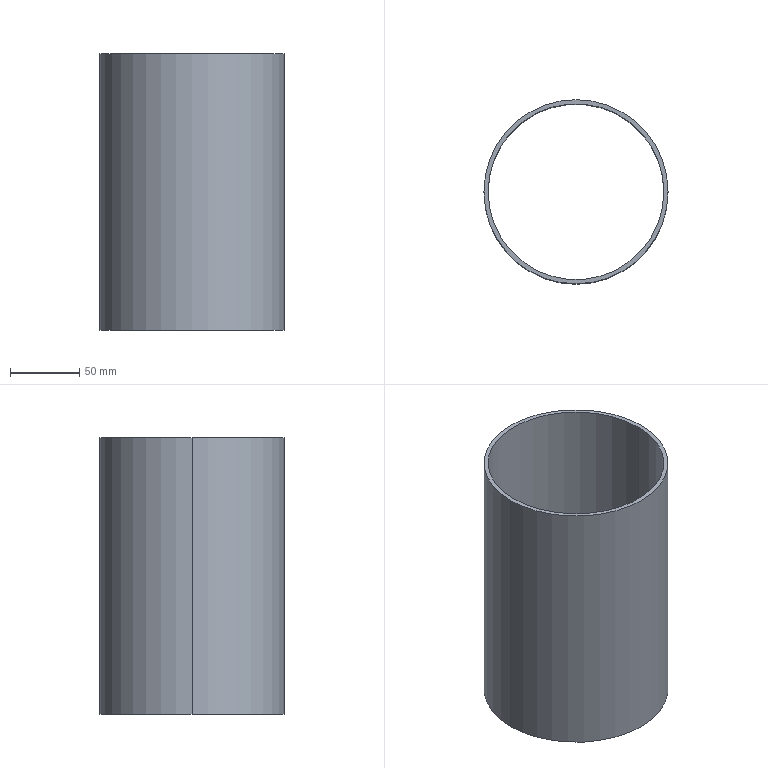Part | SolidWorks | features Extrusion 1 | 1 solid | 6 faces | box 133 x 133 x 200 mm | volume 245044 mm3 | cylinder 4 | plane 2 | commonest cylinder face diameters 127 x2 133 x2
STEP:
#1=CARTESIAN_POINT('',(-63.5,0.,200.));
#2=VERTEX_POINT('',#1);
#3=CARTESIAN_POINT('',(63.5,0.,200.));
#4=VERTEX_POINT('',#3);
#5=CARTESIAN_POINT('',(0.,0.,200.));
#6=DIRECTION('',(0.,0.,1.));
#7=DIRECTION('',(1.,0.,0.));
#8=AXIS2_PLACEMENT_3D('',#5,#6,#7);
#9=CIRCLE('',#8,63.5);
#10=EDGE_CURVE('',#2,#4,#9,.T.);
#11=ORIENTED_EDGE('',*,*,#10,.T.);
#12=CARTESIAN_POINT('',(63.5,0.,0.));
#13=VERTEX_POINT('',#12);
#14=CARTESIAN_POINT('',(63.5,0.,200.));
#15=DIRECTION('',(0.,0.,-1.));
#16=VECTOR('',#15,1000.);
#17=LINE('',#14,#16);
#18=EDGE_CURVE('',#4,#13,#17,.T.);
#19=ORIENTED_EDGE('',*,*,#18,.T.);
#20=CARTESIAN_POINT('',(-63.5,0.,0.));
#21=VERTEX_POINT('',#20);
#22=CARTESIAN_POINT('',(0.,0.,0.));
#23=DIRECTION('',(0.,0.,1.));
#24=DIRECTION('',(1.,0.,0.));
#25=AXIS2_PLACEMENT_3D('',#22,#23,#24);
#26=CIRCLE('',#25,63.5);
#27=EDGE_CURVE('',#21,#13,#26,.T.);
#28=ORIENTED_EDGE('',*,*,#27,.F.);
#29=CARTESIAN_POINT('',(-63.5,0.,200.));
#30=DIRECTION('',(0.,0.,-1.));
#31=VECTOR('',#30,1000.);
#32=LINE('',#29,#31);
#33=EDGE_CURVE('',#2,#21,#32,.T.);
#34=ORIENTED_EDGE('',*,*,#33,.F.);
#35=EDGE_LOOP('',(#11,#19,#28,#34));
#36=FACE_OUTER_BOUND('',#35,.T.);
#37=CARTESIAN_POINT('',(0.,0.,200.));
#38=DIRECTION('',(0.,0.,-1.));
#39=DIRECTION('',(-1.,0.,0.));
#40=AXIS2_PLACEMENT_3D('',#37,#38,#39);
#41=CYLINDRICAL_SURFACE('',#40,63.5);
#42=ADVANCED_FACE('',(#36),#41,.F.);
#43=CARTESIAN_POINT('',(66.5,0.,200.));
#44=VERTEX_POINT('',#43);
#45=CARTESIAN_POINT('',(-66.5,0.,200.));
#46=VERTEX_POINT('',#45);
#47=CARTESIAN_POINT('',(0.,0.,200.));
#48=DIRECTION('',(0.,0.,1.));
#49=DIRECTION('',(1.,0.,0.));
#50=AXIS2_PLACEMENT_3D('',#47,#48,#49);
#51=CIRCLE('',#50,66.5);
#52=EDGE_CURVE('',#44,#46,#51,.T.);
#53=ORIENTED_EDGE('',*,*,#52,.F.);
#54=CARTESIAN_POINT('',(66.5,0.,0.));
#55=VERTEX_POINT('',#54);
#56=CARTESIAN_POINT('',(66.5,0.,200.));
#57=DIRECTION('',(0.,0.,-1.));
#58=VECTOR('',#57,1000.);
#59=LINE('',#56,#58);
#60=EDGE_CURVE('',#44,#55,#59,.T.);
#61=ORIENTED_EDGE('',*,*,#60,.T.);
#62=CARTESIAN_POINT('',(-66.5,0.,0.));
#63=VERTEX_POINT('',#62);
#64=CARTESIAN_POINT('',(0.,0.,0.));
#65=DIRECTION('',(0.,0.,1.));
#66=DIRECTION('',(1.,0.,0.));
#67=AXIS2_PLACEMENT_3D('',#64,#65,#66);
#68=CIRCLE('',#67,66.5);
#69=EDGE_CURVE('',#55,#63,#68,.T.);
#70=ORIENTED_EDGE('',*,*,#69,.T.);
#71=CARTESIAN_POINT('',(-66.5,0.,200.));
#72=DIRECTION('',(0.,0.,-1.));
#73=VECTOR('',#72,1000.);
#74=LINE('',#71,#73);
#75=EDGE_CURVE('',#46,#63,#74,.T.);
#76=ORIENTED_EDGE('',*,*,#75,.F.);
#77=EDGE_LOOP('',(#53,#61,#70,#76));
#78=FACE_OUTER_BOUND('',#77,.T.);
#79=CARTESIAN_POINT('',(0.,0.,200.));
#80=DIRECTION('',(0.,0.,-1.));
#81=DIRECTION('',(-1.,0.,0.));
#82=AXIS2_PLACEMENT_3D('',#79,#80,#81);
#83=CYLINDRICAL_SURFACE('',#82,66.5);
#84=ADVANCED_FACE('',(#78),#83,.T.);
#85=CARTESIAN_POINT('',(0.,0.,200.));
#86=DIRECTION('',(0.,0.,1.));
#87=DIRECTION('',(1.,0.,0.));
#88=AXIS2_PLACEMENT_3D('',#85,#86,#87);
#89=CIRCLE('',#88,66.5);
#90=EDGE_CURVE('',#46,#44,#89,.T.);
#91=ORIENTED_EDGE('',*,*,#90,.T.);
#92=ORIENTED_EDGE('',*,*,#52,.T.);
#93=EDGE_LOOP('',(#91,#92));
#94=FACE_OUTER_BOUND('',#93,.T.);
#95=ORIENTED_EDGE('',*,*,#10,.F.);
#96=CARTESIAN_POINT('',(0.,0.,200.));
#97=DIRECTION('',(0.,0.,1.));
#98=DIRECTION('',(1.,0.,0.));
#99=AXIS2_PLACEMENT_3D('',#96,#97,#98);
#100=CIRCLE('',#99,63.5);
#101=EDGE_CURVE('',#4,#2,#100,.T.);
#102=ORIENTED_EDGE('',*,*,#101,.F.);
#103=EDGE_LOOP('',(#95,#102));
#104=FACE_BOUND('',#103,.T.);
#105=CARTESIAN_POINT('',(0.,0.,200.));
#106=DIRECTION('',(0.,0.,1.));
#107=DIRECTION('',(1.,0.,0.));
#108=AXIS2_PLACEMENT_3D('',#105,#106,#107);
#109=PLANE('',#108);
#110=ADVANCED_FACE('',(#94,#104),#109,.T.);
#111=CARTESIAN_POINT('',(0.,0.,0.));
#112=DIRECTION('',(0.,0.,1.));
#113=DIRECTION('',(1.,0.,0.));
#114=AXIS2_PLACEMENT_3D('',#111,#112,#113);
#115=CIRCLE('',#114,66.5);
#116=EDGE_CURVE('',#63,#55,#115,.T.);
#117=ORIENTED_EDGE('',*,*,#116,.F.);
#118=ORIENTED_EDGE('',*,*,#69,.F.);
#119=EDGE_LOOP('',(#117,#118));
#120=FACE_OUTER_BOUND('',#119,.T.);
#121=ORIENTED_EDGE('',*,*,#27,.T.);
#122=CARTESIAN_POINT('',(0.,0.,0.));
#123=DIRECTION('',(0.,0.,1.));
#124=DIRECTION('',(1.,0.,0.));
#125=AXIS2_PLACEMENT_3D('',#122,#123,#124);
#126=CIRCLE('',#125,63.5);
#127=EDGE_CURVE('',#13,#21,#126,.T.);
#128=ORIENTED_EDGE('',*,*,#127,.T.);
#129=EDGE_LOOP('',(#121,#128));
#130=FACE_BOUND('',#129,.T.);
#131=CARTESIAN_POINT('',(0.,0.,0.));
#132=DIRECTION('',(0.,0.,1.));
#133=DIRECTION('',(1.,0.,0.));
#134=AXIS2_PLACEMENT_3D('',#131,#132,#133);
#135=PLANE('',#134);
#136=ADVANCED_FACE('',(#120,#130),#135,.F.);
#137=ORIENTED_EDGE('',*,*,#60,.F.);
#138=ORIENTED_EDGE('',*,*,#90,.F.);
#139=ORIENTED_EDGE('',*,*,#75,.T.);
#140=ORIENTED_EDGE('',*,*,#116,.T.);
#141=EDGE_LOOP('',(#137,#138,#139,#140));
#142=FACE_OUTER_BOUND('',#141,.T.);
#143=CARTESIAN_POINT('',(0.,0.,200.));
#144=DIRECTION('',(0.,0.,-1.));
#145=DIRECTION('',(-1.,0.,0.));
#146=AXIS2_PLACEMENT_3D('',#143,#144,#145);
#147=CYLINDRICAL_SURFACE('',#146,66.5);
#148=ADVANCED_FACE('',(#142),#147,.T.);
#149=ORIENTED_EDGE('',*,*,#18,.F.);
#150=ORIENTED_EDGE('',*,*,#101,.T.);
#151=ORIENTED_EDGE('',*,*,#33,.T.);
#152=ORIENTED_EDGE('',*,*,#127,.F.);
#153=EDGE_LOOP('',(#149,#150,#151,#152));
#154=FACE_OUTER_BOUND('',#153,.T.);
#155=CARTESIAN_POINT('',(0.,0.,200.));
#156=DIRECTION('',(0.,0.,-1.));
#157=DIRECTION('',(-1.,0.,0.));
#158=AXIS2_PLACEMENT_3D('',#155,#156,#157);
#159=CYLINDRICAL_SURFACE('',#158,63.5);
#160=ADVANCED_FACE('',(#154),#159,.F.);
#161=CLOSED_SHELL('',(#42,#84,#110,#136,#148,#160));
#162=MANIFOLD_SOLID_BREP('',#161);
#163=CARTESIAN_POINT('',(0.,0.,0.));
#164=DIRECTION('',(0.,0.,1.));
#165=DIRECTION('',(1.,0.,0.));
#166=AXIS2_PLACEMENT_3D('',#163,#164,#165);
#167=(LENGTH_UNIT()NAMED_UNIT(*)SI_UNIT(.MILLI.,.METRE.));
#168=UNCERTAINTY_MEASURE_WITH_UNIT(LENGTH_MEASURE(0.00001),#167,'','');
#169=(NAMED_UNIT(*)PLANE_ANGLE_UNIT()SI_UNIT($,.RADIAN.));
#170=(NAMED_UNIT(*)SI_UNIT($,.STERADIAN.)SOLID_ANGLE_UNIT());
#171=(GEOMETRIC_REPRESENTATION_CONTEXT(3)GLOBAL_UNCERTAINTY_ASSIGNED_CONTEXT((#168))GLOBAL_UNIT_ASSIGNED_CONTEXT((#167,#169,#170))REPRESENTATION_CONTEXT('',''));
#172=ADVANCED_BREP_SHAPE_REPRESENTATION('',(#162,#166),#171);